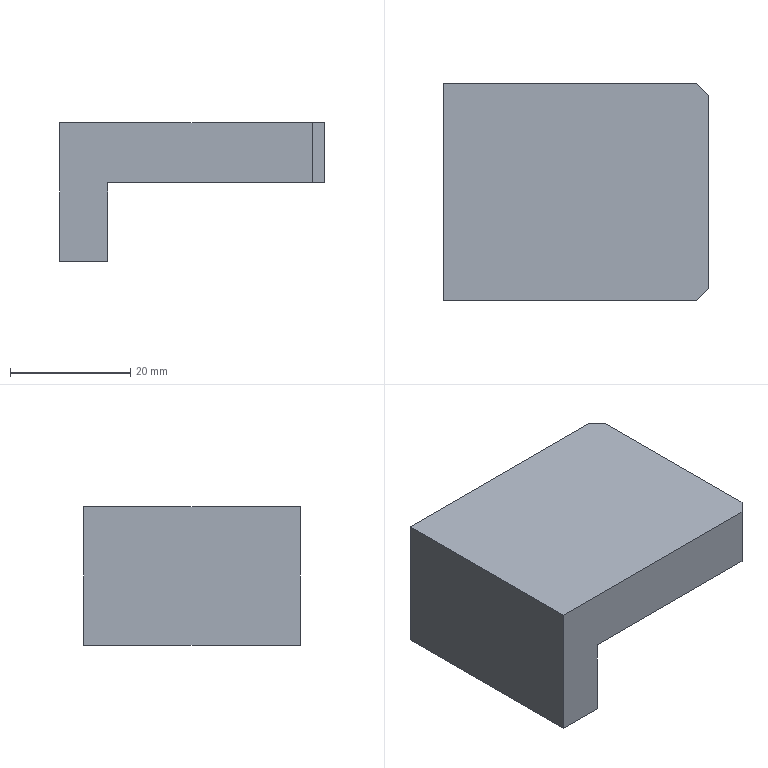Part | STEP file | Cutting plate | 1 solid | 10 faces | box 44 x 36 x 23 mm | volume 19544 mm3 | plane 10
STEP:
#1=CARTESIAN_POINT('',(0.,0.,0.));
#2=DIRECTION('',(0.,0.,1.));
#3=DIRECTION('',(1.,0.,0.));
#4=AXIS2_PLACEMENT_3D('',#1,#2,#3);
#5=CARTESIAN_POINT('',(-26.,-18.,10.));
#6=VERTEX_POINT('',#5);
#7=CARTESIAN_POINT('',(16.,-18.,10.));
#8=VERTEX_POINT('',#7);
#9=CARTESIAN_POINT('',(0.,-18.,10.));
#10=DIRECTION('',(1.,0.,0.));
#11=VECTOR('',#10,1.);
#12=LINE('',#9,#11);
#13=CARTESIAN_POINT('',(0.,0.,10.));
#14=DIRECTION('',(0.,0.,1.));
#15=DIRECTION('',(1.,0.,0.));
#16=AXIS2_PLACEMENT_3D('',#13,#14,#15);
#17=PLANE('',#16);
#18=CARTESIAN_POINT('',(0.,-18.));
#19=DIRECTION('',(1.,0.));
#20=VECTOR('',#19,1.);
#21=LINE('',#18,#20);
#22=(GEOMETRIC_REPRESENTATION_CONTEXT(2)PARAMETRIC_REPRESENTATION_CONTEXT()REPRESENTATION_CONTEXT('',''));
#23=DEFINITIONAL_REPRESENTATION('',(#21),#22);
#24=PCURVE('',#17,#23);
#25=CARTESIAN_POINT('',(-18.,-18.,10.));
#26=DIRECTION('',(0.,1.,0.));
#27=DIRECTION('',(0.,0.,1.));
#28=AXIS2_PLACEMENT_3D('',#25,#26,#27);
#29=PLANE('',#28);
#30=CARTESIAN_POINT('',(0.,18.));
#31=DIRECTION('',(0.,1.));
#32=VECTOR('',#31,1.);
#33=LINE('',#30,#32);
#34=(GEOMETRIC_REPRESENTATION_CONTEXT(2)PARAMETRIC_REPRESENTATION_CONTEXT()REPRESENTATION_CONTEXT('',''));
#35=DEFINITIONAL_REPRESENTATION('',(#33),#34);
#36=PCURVE('',#29,#35);
#37=SURFACE_CURVE('',#12,(#24,#36),.PCURVE_S1.);
#38=EDGE_CURVE('',#6,#8,#37,.T.);
#39=ORIENTED_EDGE('',*,*,#38,.T.);
#40=CARTESIAN_POINT('',(18.,-16.,10.));
#41=VERTEX_POINT('',#40);
#42=CARTESIAN_POINT('',(16.,-18.,10.));
#43=DIRECTION('',(0.7071,0.7071,0.));
#44=VECTOR('',#43,1.);
#45=LINE('',#42,#44);
#46=CARTESIAN_POINT('',(16.,-18.));
#47=DIRECTION('',(0.7071,0.7071));
#48=VECTOR('',#47,1.);
#49=LINE('',#46,#48);
#50=(GEOMETRIC_REPRESENTATION_CONTEXT(2)PARAMETRIC_REPRESENTATION_CONTEXT()REPRESENTATION_CONTEXT('',''));
#51=DEFINITIONAL_REPRESENTATION('',(#49),#50);
#52=PCURVE('',#17,#51);
#53=CARTESIAN_POINT('',(18.,-16.,10.));
#54=DIRECTION('',(-0.7071,0.7071,0.));
#55=DIRECTION('',(-0.7071,-0.7071,0.));
#56=AXIS2_PLACEMENT_3D('',#53,#54,#55);
#57=PLANE('',#56);
#58=CARTESIAN_POINT('',(2.828,0.));
#59=DIRECTION('',(-1.,0.));
#60=VECTOR('',#59,1.);
#61=LINE('',#58,#60);
#62=(GEOMETRIC_REPRESENTATION_CONTEXT(2)PARAMETRIC_REPRESENTATION_CONTEXT()REPRESENTATION_CONTEXT('',''));
#63=DEFINITIONAL_REPRESENTATION('',(#61),#62);
#64=PCURVE('',#57,#63);
#65=SURFACE_CURVE('',#45,(#52,#64),.PCURVE_S1.);
#66=EDGE_CURVE('',#8,#41,#65,.T.);
#67=ORIENTED_EDGE('',*,*,#66,.T.);
#68=CARTESIAN_POINT('',(18.,16.,10.));
#69=VERTEX_POINT('',#68);
#70=CARTESIAN_POINT('',(18.,0.,10.));
#71=DIRECTION('',(0.,1.,0.));
#72=VECTOR('',#71,1.);
#73=LINE('',#70,#72);
#74=CARTESIAN_POINT('',(18.,0.));
#75=DIRECTION('',(0.,1.));
#76=VECTOR('',#75,1.);
#77=LINE('',#74,#76);
#78=(GEOMETRIC_REPRESENTATION_CONTEXT(2)PARAMETRIC_REPRESENTATION_CONTEXT()REPRESENTATION_CONTEXT('',''));
#79=DEFINITIONAL_REPRESENTATION('',(#77),#78);
#80=PCURVE('',#17,#79);
#81=CARTESIAN_POINT('',(18.,18.,10.));
#82=DIRECTION('',(-1.,0.,0.));
#83=DIRECTION('',(0.,0.,1.));
#84=AXIS2_PLACEMENT_3D('',#81,#82,#83);
#85=PLANE('',#84);
#86=CARTESIAN_POINT('',(0.,-18.));
#87=DIRECTION('',(0.,1.));
#88=VECTOR('',#87,1.);
#89=LINE('',#86,#88);
#90=(GEOMETRIC_REPRESENTATION_CONTEXT(2)PARAMETRIC_REPRESENTATION_CONTEXT()REPRESENTATION_CONTEXT('',''));
#91=DEFINITIONAL_REPRESENTATION('',(#89),#90);
#92=PCURVE('',#85,#91);
#93=SURFACE_CURVE('',#73,(#80,#92),.PCURVE_S1.);
#94=EDGE_CURVE('',#41,#69,#93,.T.);
#95=ORIENTED_EDGE('',*,*,#94,.T.);
#96=CARTESIAN_POINT('',(16.,18.,10.));
#97=VERTEX_POINT('',#96);
#98=CARTESIAN_POINT('',(18.,16.,10.));
#99=DIRECTION('',(-0.7071,0.7071,0.));
#100=VECTOR('',#99,1.);
#101=LINE('',#98,#100);
#102=CARTESIAN_POINT('',(18.,16.));
#103=DIRECTION('',(-0.7071,0.7071));
#104=VECTOR('',#103,1.);
#105=LINE('',#102,#104);
#106=(GEOMETRIC_REPRESENTATION_CONTEXT(2)PARAMETRIC_REPRESENTATION_CONTEXT()REPRESENTATION_CONTEXT('',''));
#107=DEFINITIONAL_REPRESENTATION('',(#105),#106);
#108=PCURVE('',#17,#107);
#109=CARTESIAN_POINT('',(16.,18.,10.));
#110=DIRECTION('',(-0.7071,-0.7071,0.));
#111=DIRECTION('',(0.7071,-0.7071,0.));
#112=AXIS2_PLACEMENT_3D('',#109,#110,#111);
#113=PLANE('',#112);
#114=CARTESIAN_POINT('',(2.828,0.));
#115=DIRECTION('',(-1.,0.));
#116=VECTOR('',#115,1.);
#117=LINE('',#114,#116);
#118=(GEOMETRIC_REPRESENTATION_CONTEXT(2)PARAMETRIC_REPRESENTATION_CONTEXT()REPRESENTATION_CONTEXT('',''));
#119=DEFINITIONAL_REPRESENTATION('',(#117),#118);
#120=PCURVE('',#113,#119);
#121=SURFACE_CURVE('',#101,(#108,#120),.PCURVE_S1.);
#122=EDGE_CURVE('',#69,#97,#121,.T.);
#123=ORIENTED_EDGE('',*,*,#122,.T.);
#124=CARTESIAN_POINT('',(-26.,18.,10.));
#125=VERTEX_POINT('',#124);
#126=CARTESIAN_POINT('',(0.,18.,10.));
#127=DIRECTION('',(-1.,0.,0.));
#128=VECTOR('',#127,1.);
#129=LINE('',#126,#128);
#130=CARTESIAN_POINT('',(0.,18.));
#131=DIRECTION('',(-1.,0.));
#132=VECTOR('',#131,1.);
#133=LINE('',#130,#132);
#134=(GEOMETRIC_REPRESENTATION_CONTEXT(2)PARAMETRIC_REPRESENTATION_CONTEXT()REPRESENTATION_CONTEXT('',''));
#135=DEFINITIONAL_REPRESENTATION('',(#133),#134);
#136=PCURVE('',#17,#135);
#137=CARTESIAN_POINT('',(-18.,18.,10.));
#138=DIRECTION('',(0.,-1.,0.));
#139=DIRECTION('',(0.,0.,-1.));
#140=AXIS2_PLACEMENT_3D('',#137,#138,#139);
#141=PLANE('',#140);
#142=CARTESIAN_POINT('',(0.,18.));
#143=DIRECTION('',(0.,-1.));
#144=VECTOR('',#143,1.);
#145=LINE('',#142,#144);
#146=(GEOMETRIC_REPRESENTATION_CONTEXT(2)PARAMETRIC_REPRESENTATION_CONTEXT()REPRESENTATION_CONTEXT('',''));
#147=DEFINITIONAL_REPRESENTATION('',(#145),#146);
#148=PCURVE('',#141,#147);
#149=SURFACE_CURVE('',#129,(#136,#148),.PCURVE_S1.);
#150=EDGE_CURVE('',#97,#125,#149,.T.);
#151=ORIENTED_EDGE('',*,*,#150,.T.);
#152=CARTESIAN_POINT('',(-26.,0.,10.));
#153=DIRECTION('',(0.,-1.,0.));
#154=VECTOR('',#153,1.);
#155=LINE('',#152,#154);
#156=CARTESIAN_POINT('',(-26.,0.));
#157=DIRECTION('',(0.,-1.));
#158=VECTOR('',#157,1.);
#159=LINE('',#156,#158);
#160=(GEOMETRIC_REPRESENTATION_CONTEXT(2)PARAMETRIC_REPRESENTATION_CONTEXT()REPRESENTATION_CONTEXT('',''));
#161=DEFINITIONAL_REPRESENTATION('',(#159),#160);
#162=PCURVE('',#17,#161);
#163=CARTESIAN_POINT('',(-26.,0.,0.));
#164=DIRECTION('',(-1.,0.,0.));
#165=DIRECTION('',(0.,0.,1.));
#166=AXIS2_PLACEMENT_3D('',#163,#164,#165);
#167=PLANE('',#166);
#168=CARTESIAN_POINT('',(10.,0.));
#169=DIRECTION('',(0.,-1.));
#170=VECTOR('',#169,1.);
#171=LINE('',#168,#170);
#172=(GEOMETRIC_REPRESENTATION_CONTEXT(2)PARAMETRIC_REPRESENTATION_CONTEXT()REPRESENTATION_CONTEXT('',''));
#173=DEFINITIONAL_REPRESENTATION('',(#171),#172);
#174=PCURVE('',#167,#173);
#175=SURFACE_CURVE('',#155,(#162,#174),.PCURVE_S1.);
#176=EDGE_CURVE('',#125,#6,#175,.T.);
#177=ORIENTED_EDGE('',*,*,#176,.T.);
#178=EDGE_LOOP('',(#39,#67,#95,#123,#151,#177));
#179=FACE_BOUND('',#178,.T.);
#180=ADVANCED_FACE('',(#179),#17,.T.);
#181=CARTESIAN_POINT('',(16.,-18.,0.));
#182=VERTEX_POINT('',#181);
#183=CARTESIAN_POINT('',(16.,-18.,10.));
#184=DIRECTION('',(0.,0.,1.));
#185=VECTOR('',#184,1.);
#186=LINE('',#183,#185);
#187=CARTESIAN_POINT('',(2.828,0.));
#188=DIRECTION('',(0.,1.));
#189=VECTOR('',#188,1.);
#190=LINE('',#187,#189);
#191=(GEOMETRIC_REPRESENTATION_CONTEXT(2)PARAMETRIC_REPRESENTATION_CONTEXT()REPRESENTATION_CONTEXT('',''));
#192=DEFINITIONAL_REPRESENTATION('',(#190),#191);
#193=PCURVE('',#57,#192);
#194=CARTESIAN_POINT('',(0.,34.));
#195=DIRECTION('',(1.,0.));
#196=VECTOR('',#195,1.);
#197=LINE('',#194,#196);
#198=(GEOMETRIC_REPRESENTATION_CONTEXT(2)PARAMETRIC_REPRESENTATION_CONTEXT()REPRESENTATION_CONTEXT('',''));
#199=DEFINITIONAL_REPRESENTATION('',(#197),#198);
#200=PCURVE('',#29,#199);
#201=SURFACE_CURVE('',#186,(#193,#200),.PCURVE_S1.);
#202=EDGE_CURVE('',#182,#8,#201,.T.);
#203=ORIENTED_EDGE('',*,*,#202,.F.);
#204=CARTESIAN_POINT('',(18.,-16.,0.));
#205=VERTEX_POINT('',#204);
#206=CARTESIAN_POINT('',(18.,-16.,0.));
#207=DIRECTION('',(-0.7071,-0.7071,0.));
#208=VECTOR('',#207,1.);
#209=LINE('',#206,#208);
#210=CARTESIAN_POINT('',(0.,-10.));
#211=DIRECTION('',(1.,0.));
#212=VECTOR('',#211,1.);
#213=LINE('',#210,#212);
#214=(GEOMETRIC_REPRESENTATION_CONTEXT(2)PARAMETRIC_REPRESENTATION_CONTEXT()REPRESENTATION_CONTEXT('',''));
#215=DEFINITIONAL_REPRESENTATION('',(#213),#214);
#216=PCURVE('',#57,#215);
#217=CARTESIAN_POINT('',(0.,0.,0.));
#218=DIRECTION('',(0.,0.,1.));
#219=DIRECTION('',(1.,0.,0.));
#220=AXIS2_PLACEMENT_3D('',#217,#218,#219);
#221=PLANE('',#220);
#222=CARTESIAN_POINT('',(18.,-16.));
#223=DIRECTION('',(-0.7071,-0.7071));
#224=VECTOR('',#223,1.);
#225=LINE('',#222,#224);
#226=(GEOMETRIC_REPRESENTATION_CONTEXT(2)PARAMETRIC_REPRESENTATION_CONTEXT()REPRESENTATION_CONTEXT('',''));
#227=DEFINITIONAL_REPRESENTATION('',(#225),#226);
#228=PCURVE('',#221,#227);
#229=SURFACE_CURVE('',#209,(#216,#228),.PCURVE_S1.);
#230=EDGE_CURVE('',#205,#182,#229,.T.);
#231=ORIENTED_EDGE('',*,*,#230,.F.);
#232=CARTESIAN_POINT('',(18.,-16.,10.));
#233=DIRECTION('',(0.,0.,-1.));
#234=VECTOR('',#233,1.);
#235=LINE('',#232,#234);
#236=CARTESIAN_POINT('',(0.,0.));
#237=DIRECTION('',(0.,-1.));
#238=VECTOR('',#237,1.);
#239=LINE('',#236,#238);
#240=(GEOMETRIC_REPRESENTATION_CONTEXT(2)PARAMETRIC_REPRESENTATION_CONTEXT()REPRESENTATION_CONTEXT('',''));
#241=DEFINITIONAL_REPRESENTATION('',(#239),#240);
#242=PCURVE('',#57,#241);
#243=CARTESIAN_POINT('',(0.,-34.));
#244=DIRECTION('',(-1.,0.));
#245=VECTOR('',#244,1.);
#246=LINE('',#243,#245);
#247=(GEOMETRIC_REPRESENTATION_CONTEXT(2)PARAMETRIC_REPRESENTATION_CONTEXT()REPRESENTATION_CONTEXT('',''));
#248=DEFINITIONAL_REPRESENTATION('',(#246),#247);
#249=PCURVE('',#85,#248);
#250=SURFACE_CURVE('',#235,(#242,#249),.PCURVE_S1.);
#251=EDGE_CURVE('',#41,#205,#250,.T.);
#252=ORIENTED_EDGE('',*,*,#251,.F.);
#253=ORIENTED_EDGE('',*,*,#66,.F.);
#254=EDGE_LOOP('',(#203,#231,#252,#253));
#255=FACE_BOUND('',#254,.T.);
#256=ADVANCED_FACE('',(#255),#57,.F.);
#257=ORIENTED_EDGE('',*,*,#202,.T.);
#258=ORIENTED_EDGE('',*,*,#38,.F.);
#259=CARTESIAN_POINT('',(-26.,-18.,-13.));
#260=VERTEX_POINT('',#259);
#261=CARTESIAN_POINT('',(-26.,-18.,10.));
#262=DIRECTION('',(0.,0.,1.));
#263=VECTOR('',#262,1.);
#264=LINE('',#261,#263);
#265=CARTESIAN_POINT('',(0.,-8.));
#266=DIRECTION('',(1.,0.));
#267=VECTOR('',#266,1.);
#268=LINE('',#265,#267);
#269=(GEOMETRIC_REPRESENTATION_CONTEXT(2)PARAMETRIC_REPRESENTATION_CONTEXT()REPRESENTATION_CONTEXT('',''));
#270=DEFINITIONAL_REPRESENTATION('',(#268),#269);
#271=PCURVE('',#29,#270);
#272=CARTESIAN_POINT('',(10.,-18.));
#273=DIRECTION('',(1.,0.));
#274=VECTOR('',#273,1.);
#275=LINE('',#272,#274);
#276=(GEOMETRIC_REPRESENTATION_CONTEXT(2)PARAMETRIC_REPRESENTATION_CONTEXT()REPRESENTATION_CONTEXT('',''));
#277=DEFINITIONAL_REPRESENTATION('',(#275),#276);
#278=PCURVE('',#167,#277);
#279=SURFACE_CURVE('',#264,(#271,#278),.PCURVE_S1.);
#280=EDGE_CURVE('',#260,#6,#279,.T.);
#281=ORIENTED_EDGE('',*,*,#280,.F.);
#282=CARTESIAN_POINT('',(-18.,-18.,-13.));
#283=VERTEX_POINT('',#282);
#284=CARTESIAN_POINT('',(-18.,-18.,-13.));
#285=DIRECTION('',(-1.,0.,0.));
#286=VECTOR('',#285,1.);
#287=LINE('',#284,#286);
#288=CARTESIAN_POINT('',(-23.,0.));
#289=DIRECTION('',(0.,-1.));
#290=VECTOR('',#289,1.);
#291=LINE('',#288,#290);
#292=(GEOMETRIC_REPRESENTATION_CONTEXT(2)PARAMETRIC_REPRESENTATION_CONTEXT()REPRESENTATION_CONTEXT('',''));
#293=DEFINITIONAL_REPRESENTATION('',(#291),#292);
#294=PCURVE('',#29,#293);
#295=CARTESIAN_POINT('',(-26.,-18.,-13.));
#296=DIRECTION('',(0.,0.,1.));
#297=DIRECTION('',(1.,0.,0.));
#298=AXIS2_PLACEMENT_3D('',#295,#296,#297);
#299=PLANE('',#298);
#300=CARTESIAN_POINT('',(8.,0.));
#301=DIRECTION('',(-1.,0.));
#302=VECTOR('',#301,1.);
#303=LINE('',#300,#302);
#304=(GEOMETRIC_REPRESENTATION_CONTEXT(2)PARAMETRIC_REPRESENTATION_CONTEXT()REPRESENTATION_CONTEXT('',''));
#305=DEFINITIONAL_REPRESENTATION('',(#303),#304);
#306=PCURVE('',#299,#305);
#307=SURFACE_CURVE('',#287,(#294,#306),.PCURVE_S1.);
#308=EDGE_CURVE('',#283,#260,#307,.T.);
#309=ORIENTED_EDGE('',*,*,#308,.F.);
#310=CARTESIAN_POINT('',(-18.,-18.,0.));
#311=VERTEX_POINT('',#310);
#312=CARTESIAN_POINT('',(-18.,-18.,10.));
#313=DIRECTION('',(0.,0.,-1.));
#314=VECTOR('',#313,1.);
#315=LINE('',#312,#314);
#316=CARTESIAN_POINT('',(0.,0.));
#317=DIRECTION('',(-1.,0.));
#318=VECTOR('',#317,1.);
#319=LINE('',#316,#318);
#320=(GEOMETRIC_REPRESENTATION_CONTEXT(2)PARAMETRIC_REPRESENTATION_CONTEXT()REPRESENTATION_CONTEXT('',''));
#321=DEFINITIONAL_REPRESENTATION('',(#319),#320);
#322=PCURVE('',#29,#321);
#323=CARTESIAN_POINT('',(-18.,0.,0.));
#324=DIRECTION('',(-1.,0.,0.));
#325=DIRECTION('',(0.,0.,1.));
#326=AXIS2_PLACEMENT_3D('',#323,#324,#325);
#327=PLANE('',#326);
#328=CARTESIAN_POINT('',(10.,-18.));
#329=DIRECTION('',(-1.,0.));
#330=VECTOR('',#329,1.);
#331=LINE('',#328,#330);
#332=(GEOMETRIC_REPRESENTATION_CONTEXT(2)PARAMETRIC_REPRESENTATION_CONTEXT()REPRESENTATION_CONTEXT('',''));
#333=DEFINITIONAL_REPRESENTATION('',(#331),#332);
#334=PCURVE('',#327,#333);
#335=SURFACE_CURVE('',#315,(#322,#334),.PCURVE_S1.);
#336=EDGE_CURVE('',#311,#283,#335,.T.);
#337=ORIENTED_EDGE('',*,*,#336,.F.);
#338=CARTESIAN_POINT('',(-18.,-18.,0.));
#339=DIRECTION('',(-1.,0.,0.));
#340=VECTOR('',#339,1.);
#341=LINE('',#338,#340);
#342=CARTESIAN_POINT('',(-10.,0.));
#343=DIRECTION('',(0.,-1.));
#344=VECTOR('',#343,1.);
#345=LINE('',#342,#344);
#346=(GEOMETRIC_REPRESENTATION_CONTEXT(2)PARAMETRIC_REPRESENTATION_CONTEXT()REPRESENTATION_CONTEXT('',''));
#347=DEFINITIONAL_REPRESENTATION('',(#345),#346);
#348=PCURVE('',#29,#347);
#349=CARTESIAN_POINT('',(-18.,-18.));
#350=DIRECTION('',(-1.,0.));
#351=VECTOR('',#350,1.);
#352=LINE('',#349,#351);
#353=(GEOMETRIC_REPRESENTATION_CONTEXT(2)PARAMETRIC_REPRESENTATION_CONTEXT()REPRESENTATION_CONTEXT('',''));
#354=DEFINITIONAL_REPRESENTATION('',(#352),#353);
#355=PCURVE('',#221,#354);
#356=SURFACE_CURVE('',#341,(#348,#355),.PCURVE_S1.);
#357=EDGE_CURVE('',#182,#311,#356,.T.);
#358=ORIENTED_EDGE('',*,*,#357,.F.);
#359=EDGE_LOOP('',(#257,#258,#281,#309,#337,#358));
#360=FACE_BOUND('',#359,.T.);
#361=ADVANCED_FACE('',(#360),#29,.F.);
#362=CARTESIAN_POINT('',(-26.,18.,-13.));
#363=VERTEX_POINT('',#362);
#364=CARTESIAN_POINT('',(-26.,0.,-13.));
#365=DIRECTION('',(0.,-1.,0.));
#366=VECTOR('',#365,1.);
#367=LINE('',#364,#366);
#368=CARTESIAN_POINT('',(-13.,0.));
#369=DIRECTION('',(0.,-1.));
#370=VECTOR('',#369,1.);
#371=LINE('',#368,#370);
#372=(GEOMETRIC_REPRESENTATION_CONTEXT(2)PARAMETRIC_REPRESENTATION_CONTEXT()REPRESENTATION_CONTEXT('',''));
#373=DEFINITIONAL_REPRESENTATION('',(#371),#372);
#374=PCURVE('',#167,#373);
#375=CARTESIAN_POINT('',(0.,18.));
#376=DIRECTION('',(0.,-1.));
#377=VECTOR('',#376,1.);
#378=LINE('',#375,#377);
#379=(GEOMETRIC_REPRESENTATION_CONTEXT(2)PARAMETRIC_REPRESENTATION_CONTEXT()REPRESENTATION_CONTEXT('',''));
#380=DEFINITIONAL_REPRESENTATION('',(#378),#379);
#381=PCURVE('',#299,#380);
#382=SURFACE_CURVE('',#367,(#374,#381),.PCURVE_S1.);
#383=EDGE_CURVE('',#363,#260,#382,.T.);
#384=ORIENTED_EDGE('',*,*,#383,.T.);
#385=ORIENTED_EDGE('',*,*,#280,.T.);
#386=ORIENTED_EDGE('',*,*,#176,.F.);
#387=CARTESIAN_POINT('',(-26.,18.,0.));
#388=DIRECTION('',(0.,0.,-1.));
#389=VECTOR('',#388,1.);
#390=LINE('',#387,#389);
#391=CARTESIAN_POINT('',(0.,18.));
#392=DIRECTION('',(-1.,0.));
#393=VECTOR('',#392,1.);
#394=LINE('',#391,#393);
#395=(GEOMETRIC_REPRESENTATION_CONTEXT(2)PARAMETRIC_REPRESENTATION_CONTEXT()REPRESENTATION_CONTEXT('',''));
#396=DEFINITIONAL_REPRESENTATION('',(#394),#395);
#397=PCURVE('',#167,#396);
#398=CARTESIAN_POINT('',(10.,-8.));
#399=DIRECTION('',(1.,0.));
#400=VECTOR('',#399,1.);
#401=LINE('',#398,#400);
#402=(GEOMETRIC_REPRESENTATION_CONTEXT(2)PARAMETRIC_REPRESENTATION_CONTEXT()REPRESENTATION_CONTEXT('',''));
#403=DEFINITIONAL_REPRESENTATION('',(#401),#402);
#404=PCURVE('',#141,#403);
#405=SURFACE_CURVE('',#390,(#397,#404),.PCURVE_S1.);
#406=EDGE_CURVE('',#125,#363,#405,.T.);
#407=ORIENTED_EDGE('',*,*,#406,.T.);
#408=EDGE_LOOP('',(#384,#385,#386,#407));
#409=FACE_BOUND('',#408,.T.);
#410=ADVANCED_FACE('',(#409),#167,.T.);
#411=CARTESIAN_POINT('',(16.,18.,0.));
#412=VERTEX_POINT('',#411);
#413=CARTESIAN_POINT('',(16.,18.,10.));
#414=DIRECTION('',(0.,0.,1.));
#415=VECTOR('',#414,1.);
#416=LINE('',#413,#415);
#417=CARTESIAN_POINT('',(0.,34.));
#418=DIRECTION('',(-1.,0.));
#419=VECTOR('',#418,1.);
#420=LINE('',#417,#419);
#421=(GEOMETRIC_REPRESENTATION_CONTEXT(2)PARAMETRIC_REPRESENTATION_CONTEXT()REPRESENTATION_CONTEXT('',''));
#422=DEFINITIONAL_REPRESENTATION('',(#420),#421);
#423=PCURVE('',#141,#422);
#424=CARTESIAN_POINT('',(0.,0.));
#425=DIRECTION('',(0.,1.));
#426=VECTOR('',#425,1.);
#427=LINE('',#424,#426);
#428=(GEOMETRIC_REPRESENTATION_CONTEXT(2)PARAMETRIC_REPRESENTATION_CONTEXT()REPRESENTATION_CONTEXT('',''));
#429=DEFINITIONAL_REPRESENTATION('',(#427),#428);
#430=PCURVE('',#113,#429);
#431=SURFACE_CURVE('',#416,(#423,#430),.PCURVE_S1.);
#432=EDGE_CURVE('',#412,#97,#431,.T.);
#433=ORIENTED_EDGE('',*,*,#432,.F.);
#434=CARTESIAN_POINT('',(-18.,18.,0.));
#435=VERTEX_POINT('',#434);
#436=CARTESIAN_POINT('',(-18.,18.,0.));
#437=DIRECTION('',(1.,0.,0.));
#438=VECTOR('',#437,1.);
#439=LINE('',#436,#438);
#440=CARTESIAN_POINT('',(10.,0.));
#441=DIRECTION('',(0.,1.));
#442=VECTOR('',#441,1.);
#443=LINE('',#440,#442);
#444=(GEOMETRIC_REPRESENTATION_CONTEXT(2)PARAMETRIC_REPRESENTATION_CONTEXT()REPRESENTATION_CONTEXT('',''));
#445=DEFINITIONAL_REPRESENTATION('',(#443),#444);
#446=PCURVE('',#141,#445);
#447=CARTESIAN_POINT('',(-18.,18.));
#448=DIRECTION('',(1.,0.));
#449=VECTOR('',#448,1.);
#450=LINE('',#447,#449);
#451=(GEOMETRIC_REPRESENTATION_CONTEXT(2)PARAMETRIC_REPRESENTATION_CONTEXT()REPRESENTATION_CONTEXT('',''));
#452=DEFINITIONAL_REPRESENTATION('',(#450),#451);
#453=PCURVE('',#221,#452);
#454=SURFACE_CURVE('',#439,(#446,#453),.PCURVE_S1.);
#455=EDGE_CURVE('',#435,#412,#454,.T.);
#456=ORIENTED_EDGE('',*,*,#455,.F.);
#457=CARTESIAN_POINT('',(-18.,18.,-13.));
#458=VERTEX_POINT('',#457);
#459=CARTESIAN_POINT('',(-18.,18.,10.));
#460=DIRECTION('',(0.,0.,1.));
#461=VECTOR('',#460,1.);
#462=LINE('',#459,#461);
#463=CARTESIAN_POINT('',(0.,0.));
#464=DIRECTION('',(-1.,0.));
#465=VECTOR('',#464,1.);
#466=LINE('',#463,#465);
#467=(GEOMETRIC_REPRESENTATION_CONTEXT(2)PARAMETRIC_REPRESENTATION_CONTEXT()REPRESENTATION_CONTEXT('',''));
#468=DEFINITIONAL_REPRESENTATION('',(#466),#467);
#469=PCURVE('',#141,#468);
#470=CARTESIAN_POINT('',(10.,18.));
#471=DIRECTION('',(1.,0.));
#472=VECTOR('',#471,1.);
#473=LINE('',#470,#472);
#474=(GEOMETRIC_REPRESENTATION_CONTEXT(2)PARAMETRIC_REPRESENTATION_CONTEXT()REPRESENTATION_CONTEXT('',''));
#475=DEFINITIONAL_REPRESENTATION('',(#473),#474);
#476=PCURVE('',#327,#475);
#477=SURFACE_CURVE('',#462,(#469,#476),.PCURVE_S1.);
#478=EDGE_CURVE('',#458,#435,#477,.T.);
#479=ORIENTED_EDGE('',*,*,#478,.F.);
#480=CARTESIAN_POINT('',(-18.,18.,-13.));
#481=DIRECTION('',(1.,0.,0.));
#482=VECTOR('',#481,1.);
#483=LINE('',#480,#482);
#484=CARTESIAN_POINT('',(23.,0.));
#485=DIRECTION('',(0.,1.));
#486=VECTOR('',#485,1.);
#487=LINE('',#484,#486);
#488=(GEOMETRIC_REPRESENTATION_CONTEXT(2)PARAMETRIC_REPRESENTATION_CONTEXT()REPRESENTATION_CONTEXT('',''));
#489=DEFINITIONAL_REPRESENTATION('',(#487),#488);
#490=PCURVE('',#141,#489);
#491=CARTESIAN_POINT('',(8.,36.));
#492=DIRECTION('',(1.,0.));
#493=VECTOR('',#492,1.);
#494=LINE('',#491,#493);
#495=(GEOMETRIC_REPRESENTATION_CONTEXT(2)PARAMETRIC_REPRESENTATION_CONTEXT()REPRESENTATION_CONTEXT('',''));
#496=DEFINITIONAL_REPRESENTATION('',(#494),#495);
#497=PCURVE('',#299,#496);
#498=SURFACE_CURVE('',#483,(#490,#497),.PCURVE_S1.);
#499=EDGE_CURVE('',#363,#458,#498,.T.);
#500=ORIENTED_EDGE('',*,*,#499,.F.);
#501=ORIENTED_EDGE('',*,*,#406,.F.);
#502=ORIENTED_EDGE('',*,*,#150,.F.);
#503=EDGE_LOOP('',(#433,#456,#479,#500,#501,#502));
#504=FACE_BOUND('',#503,.T.);
#505=ADVANCED_FACE('',(#504),#141,.F.);
#506=CARTESIAN_POINT('',(18.,16.,0.));
#507=VERTEX_POINT('',#506);
#508=CARTESIAN_POINT('',(18.,16.,10.));
#509=DIRECTION('',(0.,0.,1.));
#510=VECTOR('',#509,1.);
#511=LINE('',#508,#510);
#512=CARTESIAN_POINT('',(2.828,0.));
#513=DIRECTION('',(0.,1.));
#514=VECTOR('',#513,1.);
#515=LINE('',#512,#514);
#516=(GEOMETRIC_REPRESENTATION_CONTEXT(2)PARAMETRIC_REPRESENTATION_CONTEXT()REPRESENTATION_CONTEXT('',''));
#517=DEFINITIONAL_REPRESENTATION('',(#515),#516);
#518=PCURVE('',#113,#517);
#519=CARTESIAN_POINT('',(0.,-2.));
#520=DIRECTION('',(1.,0.));
#521=VECTOR('',#520,1.);
#522=LINE('',#519,#521);
#523=(GEOMETRIC_REPRESENTATION_CONTEXT(2)PARAMETRIC_REPRESENTATION_CONTEXT()REPRESENTATION_CONTEXT('',''));
#524=DEFINITIONAL_REPRESENTATION('',(#522),#523);
#525=PCURVE('',#85,#524);
#526=SURFACE_CURVE('',#511,(#518,#525),.PCURVE_S1.);
#527=EDGE_CURVE('',#507,#69,#526,.T.);
#528=ORIENTED_EDGE('',*,*,#527,.F.);
#529=CARTESIAN_POINT('',(16.,18.,0.));
#530=DIRECTION('',(0.7071,-0.7071,0.));
#531=VECTOR('',#530,1.);
#532=LINE('',#529,#531);
#533=CARTESIAN_POINT('',(0.,-10.));
#534=DIRECTION('',(1.,0.));
#535=VECTOR('',#534,1.);
#536=LINE('',#533,#535);
#537=(GEOMETRIC_REPRESENTATION_CONTEXT(2)PARAMETRIC_REPRESENTATION_CONTEXT()REPRESENTATION_CONTEXT('',''));
#538=DEFINITIONAL_REPRESENTATION('',(#536),#537);
#539=PCURVE('',#113,#538);
#540=CARTESIAN_POINT('',(16.,18.));
#541=DIRECTION('',(0.7071,-0.7071));
#542=VECTOR('',#541,1.);
#543=LINE('',#540,#542);
#544=(GEOMETRIC_REPRESENTATION_CONTEXT(2)PARAMETRIC_REPRESENTATION_CONTEXT()REPRESENTATION_CONTEXT('',''));
#545=DEFINITIONAL_REPRESENTATION('',(#543),#544);
#546=PCURVE('',#221,#545);
#547=SURFACE_CURVE('',#532,(#539,#546),.PCURVE_S1.);
#548=EDGE_CURVE('',#412,#507,#547,.T.);
#549=ORIENTED_EDGE('',*,*,#548,.F.);
#550=ORIENTED_EDGE('',*,*,#432,.T.);
#551=ORIENTED_EDGE('',*,*,#122,.F.);
#552=EDGE_LOOP('',(#528,#549,#550,#551));
#553=FACE_BOUND('',#552,.T.);
#554=ADVANCED_FACE('',(#553),#113,.F.);
#555=ORIENTED_EDGE('',*,*,#527,.T.);
#556=ORIENTED_EDGE('',*,*,#94,.F.);
#557=ORIENTED_EDGE('',*,*,#251,.T.);
#558=CARTESIAN_POINT('',(18.,18.,0.));
#559=DIRECTION('',(0.,-1.,0.));
#560=VECTOR('',#559,1.);
#561=LINE('',#558,#560);
#562=CARTESIAN_POINT('',(-10.,0.));
#563=DIRECTION('',(0.,-1.));
#564=VECTOR('',#563,1.);
#565=LINE('',#562,#564);
#566=(GEOMETRIC_REPRESENTATION_CONTEXT(2)PARAMETRIC_REPRESENTATION_CONTEXT()REPRESENTATION_CONTEXT('',''));
#567=DEFINITIONAL_REPRESENTATION('',(#565),#566);
#568=PCURVE('',#85,#567);
#569=CARTESIAN_POINT('',(18.,18.));
#570=DIRECTION('',(0.,-1.));
#571=VECTOR('',#570,1.);
#572=LINE('',#569,#571);
#573=(GEOMETRIC_REPRESENTATION_CONTEXT(2)PARAMETRIC_REPRESENTATION_CONTEXT()REPRESENTATION_CONTEXT('',''));
#574=DEFINITIONAL_REPRESENTATION('',(#572),#573);
#575=PCURVE('',#221,#574);
#576=SURFACE_CURVE('',#561,(#568,#575),.PCURVE_S1.);
#577=EDGE_CURVE('',#507,#205,#576,.T.);
#578=ORIENTED_EDGE('',*,*,#577,.F.);
#579=EDGE_LOOP('',(#555,#556,#557,#578));
#580=FACE_BOUND('',#579,.T.);
#581=ADVANCED_FACE('',(#580),#85,.F.);
#582=ORIENTED_EDGE('',*,*,#548,.T.);
#583=ORIENTED_EDGE('',*,*,#577,.T.);
#584=ORIENTED_EDGE('',*,*,#230,.T.);
#585=ORIENTED_EDGE('',*,*,#357,.T.);
#586=CARTESIAN_POINT('',(-18.,0.,0.));
#587=DIRECTION('',(0.,-1.,0.));
#588=VECTOR('',#587,1.);
#589=LINE('',#586,#588);
#590=CARTESIAN_POINT('',(-18.,0.));
#591=DIRECTION('',(0.,-1.));
#592=VECTOR('',#591,1.);
#593=LINE('',#590,#592);
#594=(GEOMETRIC_REPRESENTATION_CONTEXT(2)PARAMETRIC_REPRESENTATION_CONTEXT()REPRESENTATION_CONTEXT('',''));
#595=DEFINITIONAL_REPRESENTATION('',(#593),#594);
#596=PCURVE('',#221,#595);
#597=CARTESIAN_POINT('',(0.,0.));
#598=DIRECTION('',(0.,-1.));
#599=VECTOR('',#598,1.);
#600=LINE('',#597,#599);
#601=(GEOMETRIC_REPRESENTATION_CONTEXT(2)PARAMETRIC_REPRESENTATION_CONTEXT()REPRESENTATION_CONTEXT('',''));
#602=DEFINITIONAL_REPRESENTATION('',(#600),#601);
#603=PCURVE('',#327,#602);
#604=SURFACE_CURVE('',#589,(#596,#603),.PCURVE_S1.);
#605=EDGE_CURVE('',#435,#311,#604,.T.);
#606=ORIENTED_EDGE('',*,*,#605,.F.);
#607=ORIENTED_EDGE('',*,*,#455,.T.);
#608=EDGE_LOOP('',(#582,#583,#584,#585,#606,#607));
#609=FACE_BOUND('',#608,.T.);
#610=ADVANCED_FACE('',(#609),#221,.F.);
#611=ORIENTED_EDGE('',*,*,#308,.T.);
#612=ORIENTED_EDGE('',*,*,#383,.F.);
#613=ORIENTED_EDGE('',*,*,#499,.T.);
#614=CARTESIAN_POINT('',(-18.,-18.,-13.));
#615=DIRECTION('',(0.,1.,0.));
#616=VECTOR('',#615,1.);
#617=LINE('',#614,#616);
#618=CARTESIAN_POINT('',(8.,0.));
#619=DIRECTION('',(0.,1.));
#620=VECTOR('',#619,1.);
#621=LINE('',#618,#620);
#622=(GEOMETRIC_REPRESENTATION_CONTEXT(2)PARAMETRIC_REPRESENTATION_CONTEXT()REPRESENTATION_CONTEXT('',''));
#623=DEFINITIONAL_REPRESENTATION('',(#621),#622);
#624=PCURVE('',#299,#623);
#625=CARTESIAN_POINT('',(-13.,-18.));
#626=DIRECTION('',(0.,1.));
#627=VECTOR('',#626,1.);
#628=LINE('',#625,#627);
#629=(GEOMETRIC_REPRESENTATION_CONTEXT(2)PARAMETRIC_REPRESENTATION_CONTEXT()REPRESENTATION_CONTEXT('',''));
#630=DEFINITIONAL_REPRESENTATION('',(#628),#629);
#631=PCURVE('',#327,#630);
#632=SURFACE_CURVE('',#617,(#624,#631),.PCURVE_S1.);
#633=EDGE_CURVE('',#283,#458,#632,.T.);
#634=ORIENTED_EDGE('',*,*,#633,.F.);
#635=EDGE_LOOP('',(#611,#612,#613,#634));
#636=FACE_BOUND('',#635,.T.);
#637=ADVANCED_FACE('',(#636),#299,.F.);
#638=ORIENTED_EDGE('',*,*,#605,.T.);
#639=ORIENTED_EDGE('',*,*,#336,.T.);
#640=ORIENTED_EDGE('',*,*,#633,.T.);
#641=ORIENTED_EDGE('',*,*,#478,.T.);
#642=EDGE_LOOP('',(#638,#639,#640,#641));
#643=FACE_BOUND('',#642,.T.);
#644=ADVANCED_FACE('',(#643),#327,.F.);
#645=CLOSED_SHELL('',(#180,#256,#361,#410,#505,#554,#581,#610,#637,#644));
#646=MANIFOLD_SOLID_BREP('',#645);
#647=(LENGTH_UNIT()NAMED_UNIT(*)SI_UNIT(.MILLI.,.METRE.));
#648=UNCERTAINTY_MEASURE_WITH_UNIT(LENGTH_MEASURE(0.0000001),#647,'','');
#649=(NAMED_UNIT(*)PLANE_ANGLE_UNIT()SI_UNIT($,.RADIAN.));
#650=(NAMED_UNIT(*)SI_UNIT($,.STERADIAN.)SOLID_ANGLE_UNIT());
#651=(GEOMETRIC_REPRESENTATION_CONTEXT(3)GLOBAL_UNCERTAINTY_ASSIGNED_CONTEXT((#648))GLOBAL_UNIT_ASSIGNED_CONTEXT((#647,#649,#650))REPRESENTATION_CONTEXT('',''));
#652=ADVANCED_BREP_SHAPE_REPRESENTATION('',(#4,#646),#651);